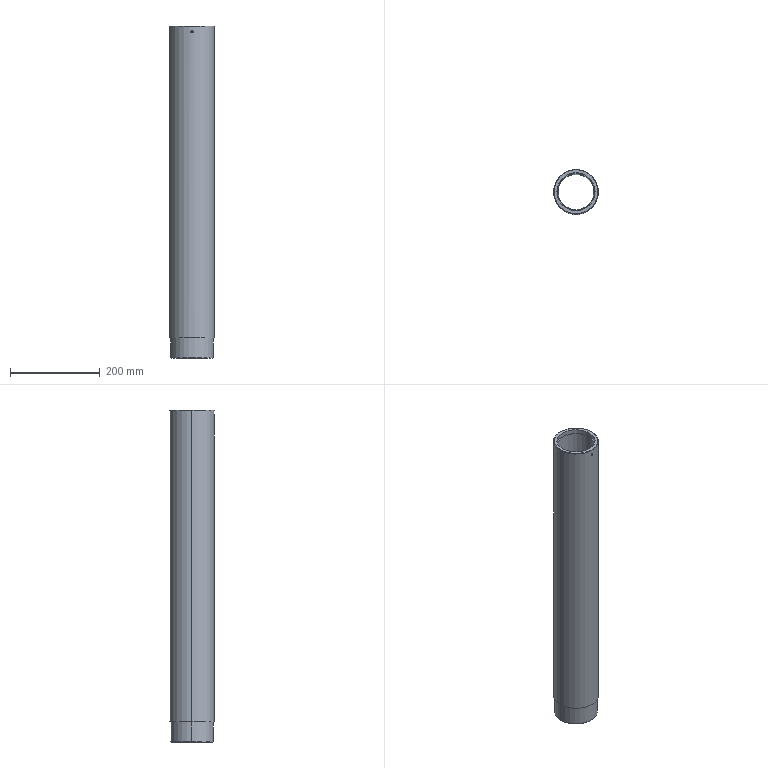Part | SolidWorks | features ICE 6, Chamfer 2, Extrusion 1, HoleWzd 1 | 1 solid | 21 faces | box 100 x 100 x 741 mm | volume 2034515 mm3 | cylinder 12 | plane 5 | cone 4 | commonest cylinder face diameters 5 x2 80 x2 83 x2 85 x2 95 x2 100 x2
STEP:
#1=CARTESIAN_POINT('',(0.,-41.5,730.5));
#2=VERTEX_POINT('',#1);
#3=CARTESIAN_POINT('',(0.,-41.5,725.5));
#4=VERTEX_POINT('',#3);
#5=CARTESIAN_POINT('',(0.,-41.5,730.5));
#6=CARTESIAN_POINT('',(-0.1631,-41.5,730.5));
#7=CARTESIAN_POINT('',(-0.3253,-41.499,730.484));
#8=CARTESIAN_POINT('',(-0.6476,-41.495,730.42));
#9=CARTESIAN_POINT('',(-0.8056,-41.492,730.372));
#10=CARTESIAN_POINT('',(-1.257,-41.482,730.185));
#11=CARTESIAN_POINT('',(-1.536,-41.472,729.999));
#12=CARTESIAN_POINT('',(-1.882,-41.457,729.654));
#13=CARTESIAN_POINT('',(-1.987,-41.452,729.525));
#14=CARTESIAN_POINT('',(-2.169,-41.443,729.254));
#15=CARTESIAN_POINT('',(-2.246,-41.439,729.11));
#16=CARTESIAN_POINT('',(-2.372,-41.432,728.808));
#17=CARTESIAN_POINT('',(-2.42,-41.429,728.649));
#18=CARTESIAN_POINT('',(-2.484,-41.426,728.329));
#19=CARTESIAN_POINT('',(-2.5,-41.425,728.167));
#20=CARTESIAN_POINT('',(-2.5,-41.425,727.837));
#21=CARTESIAN_POINT('',(-2.484,-41.426,727.674));
#22=CARTESIAN_POINT('',(-2.421,-41.429,727.355));
#23=CARTESIAN_POINT('',(-2.373,-41.432,727.196));
#24=CARTESIAN_POINT('',(-2.248,-41.439,726.893));
#25=CARTESIAN_POINT('',(-2.171,-41.443,726.749));
#26=CARTESIAN_POINT('',(-1.99,-41.452,726.478));
#27=CARTESIAN_POINT('',(-1.884,-41.457,726.349));
#28=CARTESIAN_POINT('',(-1.654,-41.467,726.118));
#29=CARTESIAN_POINT('',(-1.528,-41.472,726.015));
#30=CARTESIAN_POINT('',(-1.255,-41.481,725.832));
#31=CARTESIAN_POINT('',(-1.11,-41.485,725.754));
#32=CARTESIAN_POINT('',(-0.6586,-41.496,725.566));
#33=CARTESIAN_POINT('',(-0.3304,-41.5,725.5));
#34=CARTESIAN_POINT('',(0.,-41.5,725.5));
#35=B_SPLINE_CURVE_WITH_KNOTS('',3,(#5,#6,#7,#8,#9,#10,#11,#12,#13,#14,#15,#16,#17,#18,#19,#20,#21,#22,#23,#24,#25,#26,#27,#28,#29,#30,#31,#32,#33,#34),.UNSPECIFIED.,.F.,.F.,(4,2,2,2,2,2,2,2,2,2,2,2,2,2,4),(0.007818,0.008306,0.008795,0.009772,0.01026,0.01075,0.01124,0.01173,0.01221,0.0127,0.01319,0.01368,0.01417,0.01466,0.01563),.UNSPECIFIED.);
#36=EDGE_CURVE('',#2,#4,#35,.T.);
#37=ORIENTED_EDGE('',*,*,#36,.F.);
#38=CARTESIAN_POINT('',(0.,-50.,730.5));
#39=VERTEX_POINT('',#38);
#40=CARTESIAN_POINT('',(0.,-50.,730.5));
#41=DIRECTION('',(0.,-1.,0.));
#42=VECTOR('',#41,1000.);
#43=LINE('',#40,#42);
#44=EDGE_CURVE('',#2,#39,#43,.T.);
#45=ORIENTED_EDGE('',*,*,#44,.T.);
#46=CARTESIAN_POINT('',(0.,-50.,725.5));
#47=VERTEX_POINT('',#46);
#48=CARTESIAN_POINT('',(0.,-50.,725.5));
#49=CARTESIAN_POINT('',(-0.1652,-50.,725.5));
#50=CARTESIAN_POINT('',(-0.3277,-49.999,725.516));
#51=CARTESIAN_POINT('',(-0.6472,-49.996,725.58));
#52=CARTESIAN_POINT('',(-0.806,-49.994,725.628));
#53=CARTESIAN_POINT('',(-1.109,-49.988,725.753));
#54=CARTESIAN_POINT('',(-1.252,-49.984,725.83));
#55=CARTESIAN_POINT('',(-1.524,-49.977,726.012));
#56=CARTESIAN_POINT('',(-1.653,-49.973,726.117));
#57=CARTESIAN_POINT('',(-1.883,-49.965,726.348));
#58=CARTESIAN_POINT('',(-1.987,-49.961,726.474));
#59=CARTESIAN_POINT('',(-2.17,-49.953,726.747));
#60=CARTESIAN_POINT('',(-2.247,-49.95,726.893));
#61=CARTESIAN_POINT('',(-2.372,-49.944,727.193));
#62=CARTESIAN_POINT('',(-2.42,-49.941,727.351));
#63=CARTESIAN_POINT('',(-2.484,-49.938,727.674));
#64=CARTESIAN_POINT('',(-2.5,-49.937,727.836));
#65=CARTESIAN_POINT('',(-2.5,-49.937,728.162));
#66=CARTESIAN_POINT('',(-2.484,-49.938,728.328));
#67=CARTESIAN_POINT('',(-2.42,-49.941,728.649));
#68=CARTESIAN_POINT('',(-2.373,-49.944,728.804));
#69=CARTESIAN_POINT('',(-2.247,-49.95,729.107));
#70=CARTESIAN_POINT('',(-2.169,-49.953,729.253));
#71=CARTESIAN_POINT('',(-1.988,-49.961,729.524));
#72=CARTESIAN_POINT('',(-1.885,-49.965,729.651));
#73=CARTESIAN_POINT('',(-1.651,-49.973,729.884));
#74=CARTESIAN_POINT('',(-1.525,-49.977,729.988));
#75=CARTESIAN_POINT('',(-1.254,-49.984,730.169));
#76=CARTESIAN_POINT('',(-1.108,-49.988,730.247));
#77=CARTESIAN_POINT('',(-0.8052,-49.994,730.372));
#78=CARTESIAN_POINT('',(-0.6493,-49.996,730.42));
#79=CARTESIAN_POINT('',(-0.3289,-49.999,730.484));
#80=CARTESIAN_POINT('',(-0.1632,-50.,730.5));
#81=CARTESIAN_POINT('',(0.,-50.,730.5));
#82=B_SPLINE_CURVE_WITH_KNOTS('',3,(#48,#49,#50,#51,#52,#53,#54,#55,#56,#57,#58,#59,#60,#61,#62,#63,#64,#65,#66,#67,#68,#69,#70,#71,#72,#73,#74,#75,#76,#77,#78,#79,#80,#81),.UNSPECIFIED.,.F.,.F.,(4,2,2,2,2,2,2,2,2,2,2,2,2,2,2,2,4),(0.,0.0004886,0.0009772,0.001466,0.001954,0.002443,0.002932,0.00342,0.003909,0.004397,0.004886,0.005374,0.005863,0.006352,0.00684,0.007329,0.007817),.UNSPECIFIED.);
#83=EDGE_CURVE('',#47,#39,#82,.T.);
#84=ORIENTED_EDGE('',*,*,#83,.F.);
#85=CARTESIAN_POINT('',(0.,-50.,725.5));
#86=DIRECTION('',(0.,-1.,0.));
#87=VECTOR('',#86,1000.);
#88=LINE('',#85,#87);
#89=EDGE_CURVE('',#4,#47,#88,.T.);
#90=ORIENTED_EDGE('',*,*,#89,.F.);
#91=EDGE_LOOP('',(#37,#45,#84,#90));
#92=FACE_OUTER_BOUND('',#91,.T.);
#93=CARTESIAN_POINT('',(0.,-50.,728.));
#94=DIRECTION('',(0.,-1.,0.));
#95=DIRECTION('',(0.,0.,-1.));
#96=AXIS2_PLACEMENT_3D('',#93,#94,#95);
#97=CYLINDRICAL_SURFACE('',#96,2.5);
#98=ADVANCED_FACE('',(#92),#97,.F.);
#99=CARTESIAN_POINT('',(0.,-41.5,725.5));
#100=CARTESIAN_POINT('',(0.1652,-41.5,725.5));
#101=CARTESIAN_POINT('',(0.3277,-41.499,725.516));
#102=CARTESIAN_POINT('',(0.6473,-41.495,725.58));
#103=CARTESIAN_POINT('',(0.8061,-41.492,725.628));
#104=CARTESIAN_POINT('',(1.109,-41.485,725.753));
#105=CARTESIAN_POINT('',(1.252,-41.481,725.83));
#106=CARTESIAN_POINT('',(1.524,-41.472,726.012));
#107=CARTESIAN_POINT('',(1.653,-41.467,726.117));
#108=CARTESIAN_POINT('',(1.883,-41.457,726.348));
#109=CARTESIAN_POINT('',(1.987,-41.453,726.474));
#110=CARTESIAN_POINT('',(2.17,-41.443,726.747));
#111=CARTESIAN_POINT('',(2.247,-41.439,726.893));
#112=CARTESIAN_POINT('',(2.372,-41.432,727.193));
#113=CARTESIAN_POINT('',(2.42,-41.429,727.351));
#114=CARTESIAN_POINT('',(2.484,-41.426,727.674));
#115=CARTESIAN_POINT('',(2.5,-41.425,727.836));
#116=CARTESIAN_POINT('',(2.5,-41.425,728.162));
#117=CARTESIAN_POINT('',(2.484,-41.426,728.328));
#118=CARTESIAN_POINT('',(2.42,-41.429,728.649));
#119=CARTESIAN_POINT('',(2.373,-41.432,728.804));
#120=CARTESIAN_POINT('',(2.247,-41.439,729.107));
#121=CARTESIAN_POINT('',(2.169,-41.443,729.254));
#122=CARTESIAN_POINT('',(1.988,-41.452,729.524));
#123=CARTESIAN_POINT('',(1.885,-41.457,729.651));
#124=CARTESIAN_POINT('',(1.651,-41.467,729.884));
#125=CARTESIAN_POINT('',(1.525,-41.472,729.988));
#126=CARTESIAN_POINT('',(1.254,-41.481,730.169));
#127=CARTESIAN_POINT('',(1.108,-41.485,730.247));
#128=CARTESIAN_POINT('',(0.8052,-41.492,730.372));
#129=CARTESIAN_POINT('',(0.6493,-41.495,730.42));
#130=CARTESIAN_POINT('',(0.3289,-41.499,730.484));
#131=CARTESIAN_POINT('',(0.1632,-41.5,730.5));
#132=CARTESIAN_POINT('',(0.,-41.5,730.5));
#133=B_SPLINE_CURVE_WITH_KNOTS('',3,(#99,#100,#101,#102,#103,#104,#105,#106,#107,#108,#109,#110,#111,#112,#113,#114,#115,#116,#117,#118,#119,#120,#121,#122,#123,#124,#125,#126,#127,#128,#129,#130,#131,#132),.UNSPECIFIED.,.F.,.F.,(4,2,2,2,2,2,2,2,2,2,2,2,2,2,2,2,4),(0.,0.0004886,0.0009772,0.001466,0.001954,0.002443,0.002932,0.00342,0.003909,0.004398,0.004886,0.005375,0.005863,0.006352,0.006841,0.007329,0.007818),.UNSPECIFIED.);
#134=EDGE_CURVE('',#4,#2,#133,.T.);
#135=ORIENTED_EDGE('',*,*,#134,.T.);
#136=ORIENTED_EDGE('',*,*,#36,.T.);
#137=EDGE_LOOP('',(#135,#136));
#138=FACE_BOUND('',#137,.T.);
#139=CARTESIAN_POINT('',(-41.5,0.,681.));
#140=VERTEX_POINT('',#139);
#141=CARTESIAN_POINT('',(41.5,0.,681.));
#142=VERTEX_POINT('',#141);
#143=CARTESIAN_POINT('',(0.,0.,681.));
#144=DIRECTION('',(0.,0.,1.));
#145=DIRECTION('',(1.,0.,0.));
#146=AXIS2_PLACEMENT_3D('',#143,#144,#145);
#147=CIRCLE('',#146,41.5);
#148=EDGE_CURVE('',#140,#142,#147,.T.);
#149=ORIENTED_EDGE('',*,*,#148,.F.);
#150=CARTESIAN_POINT('',(-41.5,0.,731.));
#151=VERTEX_POINT('',#150);
#152=CARTESIAN_POINT('',(-41.5,0.,681.));
#153=DIRECTION('',(0.,0.,1.));
#154=VECTOR('',#153,1000.);
#155=LINE('',#152,#154);
#156=EDGE_CURVE('',#140,#151,#155,.T.);
#157=ORIENTED_EDGE('',*,*,#156,.T.);
#158=CARTESIAN_POINT('',(41.5,0.,731.));
#159=VERTEX_POINT('',#158);
#160=CARTESIAN_POINT('',(0.,0.,731.));
#161=DIRECTION('',(0.,0.,1.));
#162=DIRECTION('',(1.,0.,0.));
#163=AXIS2_PLACEMENT_3D('',#160,#161,#162);
#164=CIRCLE('',#163,41.5);
#165=EDGE_CURVE('',#151,#159,#164,.T.);
#166=ORIENTED_EDGE('',*,*,#165,.T.);
#167=CARTESIAN_POINT('',(41.5,0.,681.));
#168=DIRECTION('',(0.,0.,1.));
#169=VECTOR('',#168,1000.);
#170=LINE('',#167,#169);
#171=EDGE_CURVE('',#142,#159,#170,.T.);
#172=ORIENTED_EDGE('',*,*,#171,.F.);
#173=EDGE_LOOP('',(#149,#157,#166,#172));
#174=FACE_OUTER_BOUND('',#173,.T.);
#175=CARTESIAN_POINT('',(0.,0.,681.));
#176=DIRECTION('',(0.,0.,1.));
#177=DIRECTION('',(1.,0.,0.));
#178=AXIS2_PLACEMENT_3D('',#175,#176,#177);
#179=CYLINDRICAL_SURFACE('',#178,41.5);
#180=ADVANCED_FACE('',(#138,#174),#179,.F.);
#181=CARTESIAN_POINT('',(-42.5,0.,731.));
#182=VERTEX_POINT('',#181);
#183=CARTESIAN_POINT('',(42.5,0.,731.));
#184=VERTEX_POINT('',#183);
#185=CARTESIAN_POINT('',(0.,0.,731.));
#186=DIRECTION('',(0.,0.,1.));
#187=DIRECTION('',(1.,0.,0.));
#188=AXIS2_PLACEMENT_3D('',#185,#186,#187);
#189=CIRCLE('',#188,42.5);
#190=EDGE_CURVE('',#182,#184,#189,.T.);
#191=ORIENTED_EDGE('',*,*,#190,.F.);
#192=CARTESIAN_POINT('',(-42.5,0.,741.));
#193=VERTEX_POINT('',#192);
#194=CARTESIAN_POINT('',(-42.5,0.,731.));
#195=DIRECTION('',(0.,0.,1.));
#196=VECTOR('',#195,1000.);
#197=LINE('',#194,#196);
#198=EDGE_CURVE('',#182,#193,#197,.T.);
#199=ORIENTED_EDGE('',*,*,#198,.T.);
#200=CARTESIAN_POINT('',(42.5,0.,741.));
#201=VERTEX_POINT('',#200);
#202=CARTESIAN_POINT('',(0.,0.,741.));
#203=DIRECTION('',(0.,0.,1.));
#204=DIRECTION('',(1.,0.,0.));
#205=AXIS2_PLACEMENT_3D('',#202,#203,#204);
#206=CIRCLE('',#205,42.5);
#207=EDGE_CURVE('',#193,#201,#206,.T.);
#208=ORIENTED_EDGE('',*,*,#207,.T.);
#209=CARTESIAN_POINT('',(42.5,0.,731.));
#210=DIRECTION('',(0.,0.,1.));
#211=VECTOR('',#210,1000.);
#212=LINE('',#209,#211);
#213=EDGE_CURVE('',#184,#201,#212,.T.);
#214=ORIENTED_EDGE('',*,*,#213,.F.);
#215=EDGE_LOOP('',(#191,#199,#208,#214));
#216=FACE_OUTER_BOUND('',#215,.T.);
#217=CARTESIAN_POINT('',(0.,0.,731.));
#218=DIRECTION('',(0.,0.,1.));
#219=DIRECTION('',(1.,0.,0.));
#220=AXIS2_PLACEMENT_3D('',#217,#218,#219);
#221=CYLINDRICAL_SURFACE('',#220,42.5);
#222=ADVANCED_FACE('',(#216),#221,.F.);
#223=CARTESIAN_POINT('',(49.,0.,741.));
#224=VERTEX_POINT('',#223);
#225=CARTESIAN_POINT('',(-49.,0.,741.));
#226=VERTEX_POINT('',#225);
#227=CARTESIAN_POINT('',(0.,0.,741.));
#228=DIRECTION('',(0.,0.,1.));
#229=DIRECTION('',(1.,0.,0.));
#230=AXIS2_PLACEMENT_3D('',#227,#228,#229);
#231=CIRCLE('',#230,49.);
#232=EDGE_CURVE('',#224,#226,#231,.T.);
#233=ORIENTED_EDGE('',*,*,#232,.F.);
#234=CARTESIAN_POINT('',(50.,0.,740.));
#235=VERTEX_POINT('',#234);
#236=CARTESIAN_POINT('',(49.,0.,741.));
#237=DIRECTION('',(0.7071,0.,-0.7071));
#238=VECTOR('',#237,1000.);
#239=LINE('',#236,#238);
#240=EDGE_CURVE('',#224,#235,#239,.T.);
#241=ORIENTED_EDGE('',*,*,#240,.T.);
#242=CARTESIAN_POINT('',(-50.,0.,740.));
#243=VERTEX_POINT('',#242);
#244=CARTESIAN_POINT('',(0.,0.,740.));
#245=DIRECTION('',(0.,0.,-1.));
#246=DIRECTION('',(1.,0.,0.));
#247=AXIS2_PLACEMENT_3D('',#244,#245,#246);
#248=CIRCLE('',#247,50.);
#249=EDGE_CURVE('',#243,#235,#248,.T.);
#250=ORIENTED_EDGE('',*,*,#249,.F.);
#251=CARTESIAN_POINT('',(-49.,0.,741.));
#252=DIRECTION('',(-0.7071,0.,-0.7071));
#253=VECTOR('',#252,1000.);
#254=LINE('',#251,#253);
#255=EDGE_CURVE('',#226,#243,#254,.T.);
#256=ORIENTED_EDGE('',*,*,#255,.F.);
#257=EDGE_LOOP('',(#233,#241,#250,#256));
#258=FACE_OUTER_BOUND('',#257,.T.);
#259=CARTESIAN_POINT('',(0.,0.,741.));
#260=DIRECTION('',(0.,0.,-1.));
#261=DIRECTION('',(-1.,0.,0.));
#262=AXIS2_PLACEMENT_3D('',#259,#260,#261);
#263=CONICAL_SURFACE('',#262,49.,0.7854);
#264=ADVANCED_FACE('',(#258),#263,.T.);
#265=CARTESIAN_POINT('',(-46.5,0.,0.));
#266=VERTEX_POINT('',#265);
#267=CARTESIAN_POINT('',(46.5,0.,0.));
#268=VERTEX_POINT('',#267);
#269=CARTESIAN_POINT('',(0.,0.,0.));
#270=DIRECTION('',(0.,0.,-1.));
#271=DIRECTION('',(1.,0.,0.));
#272=AXIS2_PLACEMENT_3D('',#269,#270,#271);
#273=CIRCLE('',#272,46.5);
#274=EDGE_CURVE('',#266,#268,#273,.T.);
#275=ORIENTED_EDGE('',*,*,#274,.F.);
#276=CARTESIAN_POINT('',(-47.5,0.,1.));
#277=VERTEX_POINT('',#276);
#278=CARTESIAN_POINT('',(-46.5,0.,0.));
#279=DIRECTION('',(-0.7071,0.,0.7071));
#280=VECTOR('',#279,1000.);
#281=LINE('',#278,#280);
#282=EDGE_CURVE('',#266,#277,#281,.T.);
#283=ORIENTED_EDGE('',*,*,#282,.T.);
#284=CARTESIAN_POINT('',(47.5,0.,1.));
#285=VERTEX_POINT('',#284);
#286=CARTESIAN_POINT('',(0.,0.,1.));
#287=DIRECTION('',(0.,0.,1.));
#288=DIRECTION('',(1.,0.,0.));
#289=AXIS2_PLACEMENT_3D('',#286,#287,#288);
#290=CIRCLE('',#289,47.5);
#291=EDGE_CURVE('',#285,#277,#290,.T.);
#292=ORIENTED_EDGE('',*,*,#291,.F.);
#293=CARTESIAN_POINT('',(46.5,0.,0.));
#294=DIRECTION('',(0.7071,0.,0.7071));
#295=VECTOR('',#294,1000.);
#296=LINE('',#293,#295);
#297=EDGE_CURVE('',#268,#285,#296,.T.);
#298=ORIENTED_EDGE('',*,*,#297,.F.);
#299=EDGE_LOOP('',(#275,#283,#292,#298));
#300=FACE_OUTER_BOUND('',#299,.T.);
#301=CARTESIAN_POINT('',(0.,0.,0.));
#302=DIRECTION('',(0.,0.,1.));
#303=DIRECTION('',(1.,0.,0.));
#304=AXIS2_PLACEMENT_3D('',#301,#302,#303);
#305=CONICAL_SURFACE('',#304,46.5,0.7854);
#306=ADVANCED_FACE('',(#300),#305,.T.);
#307=CARTESIAN_POINT('',(-47.5,0.,45.));
#308=VERTEX_POINT('',#307);
#309=CARTESIAN_POINT('',(47.5,0.,45.));
#310=VERTEX_POINT('',#309);
#311=CARTESIAN_POINT('',(0.,0.,45.));
#312=DIRECTION('',(0.,0.,-1.));
#313=DIRECTION('',(-1.,0.,0.));
#314=AXIS2_PLACEMENT_3D('',#311,#312,#313);
#315=CIRCLE('',#314,47.5);
#316=EDGE_CURVE('',#308,#310,#315,.T.);
#317=ORIENTED_EDGE('',*,*,#316,.T.);
#318=CARTESIAN_POINT('',(47.5,0.,45.));
#319=DIRECTION('',(0.,0.,-1.));
#320=VECTOR('',#319,1000.);
#321=LINE('',#318,#320);
#322=EDGE_CURVE('',#310,#285,#321,.T.);
#323=ORIENTED_EDGE('',*,*,#322,.T.);
#324=ORIENTED_EDGE('',*,*,#291,.T.);
#325=CARTESIAN_POINT('',(-47.5,0.,45.));
#326=DIRECTION('',(0.,0.,-1.));
#327=VECTOR('',#326,1000.);
#328=LINE('',#325,#327);
#329=EDGE_CURVE('',#308,#277,#328,.T.);
#330=ORIENTED_EDGE('',*,*,#329,.F.);
#331=EDGE_LOOP('',(#317,#323,#324,#330));
#332=FACE_OUTER_BOUND('',#331,.T.);
#333=CARTESIAN_POINT('',(0.,0.,45.));
#334=DIRECTION('',(0.,0.,-1.));
#335=DIRECTION('',(-1.,0.,0.));
#336=AXIS2_PLACEMENT_3D('',#333,#334,#335);
#337=CYLINDRICAL_SURFACE('',#336,47.5);
#338=ADVANCED_FACE('',(#332),#337,.T.);
#339=ORIENTED_EDGE('',*,*,#249,.T.);
#340=CARTESIAN_POINT('',(50.,0.,45.));
#341=VERTEX_POINT('',#340);
#342=CARTESIAN_POINT('',(50.,0.,741.));
#343=DIRECTION('',(0.,0.,-1.));
#344=VECTOR('',#343,1000.);
#345=LINE('',#342,#344);
#346=EDGE_CURVE('',#235,#341,#345,.T.);
#347=ORIENTED_EDGE('',*,*,#346,.T.);
#348=CARTESIAN_POINT('',(-50.,0.,45.));
#349=VERTEX_POINT('',#348);
#350=CARTESIAN_POINT('',(0.,0.,45.));
#351=DIRECTION('',(0.,0.,-1.));
#352=DIRECTION('',(-1.,0.,0.));
#353=AXIS2_PLACEMENT_3D('',#350,#351,#352);
#354=CIRCLE('',#353,50.);
#355=EDGE_CURVE('',#349,#341,#354,.T.);
#356=ORIENTED_EDGE('',*,*,#355,.F.);
#357=CARTESIAN_POINT('',(-50.,0.,741.));
#358=DIRECTION('',(0.,0.,-1.));
#359=VECTOR('',#358,1000.);
#360=LINE('',#357,#359);
#361=EDGE_CURVE('',#243,#349,#360,.T.);
#362=ORIENTED_EDGE('',*,*,#361,.F.);
#363=EDGE_LOOP('',(#339,#347,#356,#362));
#364=FACE_OUTER_BOUND('',#363,.T.);
#365=CARTESIAN_POINT('',(0.,0.,741.));
#366=DIRECTION('',(0.,0.,-1.));
#367=DIRECTION('',(-1.,0.,0.));
#368=AXIS2_PLACEMENT_3D('',#365,#366,#367);
#369=CYLINDRICAL_SURFACE('',#368,50.);
#370=ADVANCED_FACE('',(#364),#369,.T.);
#371=CARTESIAN_POINT('',(-40.,0.,681.));
#372=VERTEX_POINT('',#371);
#373=CARTESIAN_POINT('',(40.,0.,681.));
#374=VERTEX_POINT('',#373);
#375=CARTESIAN_POINT('',(0.,0.,681.));
#376=DIRECTION('',(0.,0.,1.));
#377=DIRECTION('',(1.,0.,0.));
#378=AXIS2_PLACEMENT_3D('',#375,#376,#377);
#379=CIRCLE('',#378,40.);
#380=EDGE_CURVE('',#372,#374,#379,.T.);
#381=ORIENTED_EDGE('',*,*,#380,.T.);
#382=CARTESIAN_POINT('',(40.,0.,0.));
#383=VERTEX_POINT('',#382);
#384=CARTESIAN_POINT('',(40.,0.,741.));
#385=DIRECTION('',(0.,0.,-1.));
#386=VECTOR('',#385,1000.);
#387=LINE('',#384,#386);
#388=EDGE_CURVE('',#374,#383,#387,.T.);
#389=ORIENTED_EDGE('',*,*,#388,.T.);
#390=CARTESIAN_POINT('',(-40.,0.,0.));
#391=VERTEX_POINT('',#390);
#392=CARTESIAN_POINT('',(0.,0.,0.));
#393=DIRECTION('',(0.,0.,1.));
#394=DIRECTION('',(1.,0.,0.));
#395=AXIS2_PLACEMENT_3D('',#392,#393,#394);
#396=CIRCLE('',#395,40.);
#397=EDGE_CURVE('',#391,#383,#396,.T.);
#398=ORIENTED_EDGE('',*,*,#397,.F.);
#399=CARTESIAN_POINT('',(-40.,0.,741.));
#400=DIRECTION('',(0.,0.,-1.));
#401=VECTOR('',#400,1000.);
#402=LINE('',#399,#401);
#403=EDGE_CURVE('',#372,#391,#402,.T.);
#404=ORIENTED_EDGE('',*,*,#403,.F.);
#405=EDGE_LOOP('',(#381,#389,#398,#404));
#406=FACE_OUTER_BOUND('',#405,.T.);
#407=CARTESIAN_POINT('',(0.,0.,741.));
#408=DIRECTION('',(0.,0.,-1.));
#409=DIRECTION('',(-1.,0.,0.));
#410=AXIS2_PLACEMENT_3D('',#407,#408,#409);
#411=CYLINDRICAL_SURFACE('',#410,40.);
#412=ADVANCED_FACE('',(#406),#411,.F.);
#413=ORIENTED_EDGE('',*,*,#388,.F.);
#414=CARTESIAN_POINT('',(0.,0.,681.));
#415=DIRECTION('',(0.,0.,1.));
#416=DIRECTION('',(1.,0.,0.));
#417=AXIS2_PLACEMENT_3D('',#414,#415,#416);
#418=CIRCLE('',#417,40.);
#419=EDGE_CURVE('',#374,#372,#418,.T.);
#420=ORIENTED_EDGE('',*,*,#419,.T.);
#421=ORIENTED_EDGE('',*,*,#403,.T.);
#422=CARTESIAN_POINT('',(0.,0.,0.));
#423=DIRECTION('',(0.,0.,1.));
#424=DIRECTION('',(1.,0.,0.));
#425=AXIS2_PLACEMENT_3D('',#422,#423,#424);
#426=CIRCLE('',#425,40.);
#427=EDGE_CURVE('',#383,#391,#426,.T.);
#428=ORIENTED_EDGE('',*,*,#427,.F.);
#429=EDGE_LOOP('',(#413,#420,#421,#428));
#430=FACE_OUTER_BOUND('',#429,.T.);
#431=CARTESIAN_POINT('',(0.,0.,741.));
#432=DIRECTION('',(0.,0.,-1.));
#433=DIRECTION('',(-1.,0.,0.));
#434=AXIS2_PLACEMENT_3D('',#431,#432,#433);
#435=CYLINDRICAL_SURFACE('',#434,40.);
#436=ADVANCED_FACE('',(#430),#435,.F.);
#437=CARTESIAN_POINT('',(0.,0.,0.));
#438=DIRECTION('',(0.,0.,-1.));
#439=DIRECTION('',(1.,0.,0.));
#440=AXIS2_PLACEMENT_3D('',#437,#438,#439);
#441=CIRCLE('',#440,46.5);
#442=EDGE_CURVE('',#268,#266,#441,.T.);
#443=ORIENTED_EDGE('',*,*,#442,.T.);
#444=ORIENTED_EDGE('',*,*,#274,.T.);
#445=EDGE_LOOP('',(#443,#444));
#446=FACE_OUTER_BOUND('',#445,.T.);
#447=ORIENTED_EDGE('',*,*,#397,.T.);
#448=ORIENTED_EDGE('',*,*,#427,.T.);
#449=EDGE_LOOP('',(#447,#448));
#450=FACE_BOUND('',#449,.T.);
#451=CARTESIAN_POINT('',(0.,0.,0.));
#452=DIRECTION('',(0.,0.,1.));
#453=DIRECTION('',(1.,0.,0.));
#454=AXIS2_PLACEMENT_3D('',#451,#452,#453);
#455=PLANE('',#454);
#456=ADVANCED_FACE('',(#446,#450),#455,.F.);
#457=ORIENTED_EDGE('',*,*,#346,.F.);
#458=CARTESIAN_POINT('',(0.,0.,740.));
#459=DIRECTION('',(0.,0.,-1.));
#460=DIRECTION('',(1.,0.,0.));
#461=AXIS2_PLACEMENT_3D('',#458,#459,#460);
#462=CIRCLE('',#461,50.);
#463=EDGE_CURVE('',#235,#243,#462,.T.);
#464=ORIENTED_EDGE('',*,*,#463,.T.);
#465=ORIENTED_EDGE('',*,*,#361,.T.);
#466=CARTESIAN_POINT('',(0.,0.,45.));
#467=DIRECTION('',(0.,0.,-1.));
#468=DIRECTION('',(-1.,0.,0.));
#469=AXIS2_PLACEMENT_3D('',#466,#467,#468);
#470=CIRCLE('',#469,50.);
#471=EDGE_CURVE('',#341,#349,#470,.T.);
#472=ORIENTED_EDGE('',*,*,#471,.F.);
#473=EDGE_LOOP('',(#457,#464,#465,#472));
#474=FACE_OUTER_BOUND('',#473,.T.);
#475=ORIENTED_EDGE('',*,*,#83,.T.);
#476=CARTESIAN_POINT('',(0.,-50.,730.5));
#477=CARTESIAN_POINT('',(0.1631,-50.,730.5));
#478=CARTESIAN_POINT('',(0.3253,-49.999,730.484));
#479=CARTESIAN_POINT('',(0.6476,-49.996,730.42));
#480=CARTESIAN_POINT('',(0.8056,-49.994,730.372));
#481=CARTESIAN_POINT('',(1.257,-49.985,730.185));
#482=CARTESIAN_POINT('',(1.536,-49.977,729.999));
#483=CARTESIAN_POINT('',(1.882,-49.965,729.654));
#484=CARTESIAN_POINT('',(1.987,-49.961,729.525));
#485=CARTESIAN_POINT('',(2.169,-49.953,729.254));
#486=CARTESIAN_POINT('',(2.246,-49.95,729.11));
#487=CARTESIAN_POINT('',(2.372,-49.944,728.808));
#488=CARTESIAN_POINT('',(2.42,-49.941,728.649));
#489=CARTESIAN_POINT('',(2.484,-49.938,728.329));
#490=CARTESIAN_POINT('',(2.5,-49.937,728.167));
#491=CARTESIAN_POINT('',(2.5,-49.937,727.837));
#492=CARTESIAN_POINT('',(2.484,-49.938,727.674));
#493=CARTESIAN_POINT('',(2.421,-49.941,727.355));
#494=CARTESIAN_POINT('',(2.373,-49.944,727.196));
#495=CARTESIAN_POINT('',(2.248,-49.949,726.893));
#496=CARTESIAN_POINT('',(2.171,-49.953,726.749));
#497=CARTESIAN_POINT('',(1.99,-49.96,726.478));
#498=CARTESIAN_POINT('',(1.884,-49.965,726.349));
#499=CARTESIAN_POINT('',(1.654,-49.973,726.118));
#500=CARTESIAN_POINT('',(1.528,-49.977,726.015));
#501=CARTESIAN_POINT('',(1.255,-49.984,725.832));
#502=CARTESIAN_POINT('',(1.11,-49.988,725.754));
#503=CARTESIAN_POINT('',(0.6585,-49.997,725.566));
#504=CARTESIAN_POINT('',(0.3303,-50.,725.5));
#505=CARTESIAN_POINT('',(0.,-50.,725.5));
#506=B_SPLINE_CURVE_WITH_KNOTS('',3,(#476,#477,#478,#479,#480,#481,#482,#483,#484,#485,#486,#487,#488,#489,#490,#491,#492,#493,#494,#495,#496,#497,#498,#499,#500,#501,#502,#503,#504,#505),.UNSPECIFIED.,.F.,.F.,(4,2,2,2,2,2,2,2,2,2,2,2,2,2,4),(0.007817,0.008306,0.008794,0.009771,0.01026,0.01075,0.01124,0.01173,0.01221,0.0127,0.01319,0.01368,0.01417,0.01466,0.01563),.UNSPECIFIED.);
#507=EDGE_CURVE('',#39,#47,#506,.T.);
#508=ORIENTED_EDGE('',*,*,#507,.T.);
#509=EDGE_LOOP('',(#475,#508));
#510=FACE_BOUND('',#509,.T.);
#511=CARTESIAN_POINT('',(0.,0.,741.));
#512=DIRECTION('',(0.,0.,-1.));
#513=DIRECTION('',(-1.,0.,0.));
#514=AXIS2_PLACEMENT_3D('',#511,#512,#513);
#515=CYLINDRICAL_SURFACE('',#514,50.);
#516=ADVANCED_FACE('',(#474,#510),#515,.T.);
#517=CARTESIAN_POINT('',(0.,0.,741.));
#518=DIRECTION('',(0.,0.,1.));
#519=DIRECTION('',(1.,0.,0.));
#520=AXIS2_PLACEMENT_3D('',#517,#518,#519);
#521=CIRCLE('',#520,42.5);
#522=EDGE_CURVE('',#201,#193,#521,.T.);
#523=ORIENTED_EDGE('',*,*,#522,.F.);
#524=ORIENTED_EDGE('',*,*,#207,.F.);
#525=EDGE_LOOP('',(#523,#524));
#526=FACE_BOUND('',#525,.T.);
#527=CARTESIAN_POINT('',(0.,0.,741.));
#528=DIRECTION('',(0.,0.,1.));
#529=DIRECTION('',(1.,0.,0.));
#530=AXIS2_PLACEMENT_3D('',#527,#528,#529);
#531=CIRCLE('',#530,49.);
#532=EDGE_CURVE('',#226,#224,#531,.T.);
#533=ORIENTED_EDGE('',*,*,#532,.T.);
#534=ORIENTED_EDGE('',*,*,#232,.T.);
#535=EDGE_LOOP('',(#533,#534));
#536=FACE_OUTER_BOUND('',#535,.T.);
#537=CARTESIAN_POINT('',(0.,0.,741.));
#538=DIRECTION('',(0.,0.,1.));
#539=DIRECTION('',(1.,0.,0.));
#540=AXIS2_PLACEMENT_3D('',#537,#538,#539);
#541=PLANE('',#540);
#542=ADVANCED_FACE('',(#526,#536),#541,.T.);
#543=ORIENTED_EDGE('',*,*,#316,.F.);
#544=CARTESIAN_POINT('',(0.,0.,45.));
#545=DIRECTION('',(0.,0.,-1.));
#546=DIRECTION('',(-1.,0.,0.));
#547=AXIS2_PLACEMENT_3D('',#544,#545,#546);
#548=CIRCLE('',#547,47.5);
#549=EDGE_CURVE('',#310,#308,#548,.T.);
#550=ORIENTED_EDGE('',*,*,#549,.F.);
#551=EDGE_LOOP('',(#543,#550));
#552=FACE_BOUND('',#551,.T.);
#553=ORIENTED_EDGE('',*,*,#355,.T.);
#554=ORIENTED_EDGE('',*,*,#471,.T.);
#555=EDGE_LOOP('',(#553,#554));
#556=FACE_OUTER_BOUND('',#555,.T.);
#557=CARTESIAN_POINT('',(0.,0.,45.));
#558=DIRECTION('',(0.,0.,-1.));
#559=DIRECTION('',(-1.,0.,0.));
#560=AXIS2_PLACEMENT_3D('',#557,#558,#559);
#561=PLANE('',#560);
#562=ADVANCED_FACE('',(#552,#556),#561,.T.);
#563=ORIENTED_EDGE('',*,*,#322,.F.);
#564=ORIENTED_EDGE('',*,*,#549,.T.);
#565=ORIENTED_EDGE('',*,*,#329,.T.);
#566=CARTESIAN_POINT('',(0.,0.,1.));
#567=DIRECTION('',(0.,0.,1.));
#568=DIRECTION('',(1.,0.,0.));
#569=AXIS2_PLACEMENT_3D('',#566,#567,#568);
#570=CIRCLE('',#569,47.5);
#571=EDGE_CURVE('',#277,#285,#570,.T.);
#572=ORIENTED_EDGE('',*,*,#571,.T.);
#573=EDGE_LOOP('',(#563,#564,#565,#572));
#574=FACE_OUTER_BOUND('',#573,.T.);
#575=CARTESIAN_POINT('',(0.,0.,45.));
#576=DIRECTION('',(0.,0.,-1.));
#577=DIRECTION('',(-1.,0.,0.));
#578=AXIS2_PLACEMENT_3D('',#575,#576,#577);
#579=CYLINDRICAL_SURFACE('',#578,47.5);
#580=ADVANCED_FACE('',(#574),#579,.T.);
#581=ORIENTED_EDGE('',*,*,#282,.F.);
#582=ORIENTED_EDGE('',*,*,#442,.F.);
#583=ORIENTED_EDGE('',*,*,#297,.T.);
#584=ORIENTED_EDGE('',*,*,#571,.F.);
#585=EDGE_LOOP('',(#581,#582,#583,#584));
#586=FACE_OUTER_BOUND('',#585,.T.);
#587=CARTESIAN_POINT('',(0.,0.,0.));
#588=DIRECTION('',(0.,0.,1.));
#589=DIRECTION('',(1.,0.,0.));
#590=AXIS2_PLACEMENT_3D('',#587,#588,#589);
#591=CONICAL_SURFACE('',#590,46.5,0.7854);
#592=ADVANCED_FACE('',(#586),#591,.T.);
#593=ORIENTED_EDGE('',*,*,#240,.F.);
#594=ORIENTED_EDGE('',*,*,#532,.F.);
#595=ORIENTED_EDGE('',*,*,#255,.T.);
#596=ORIENTED_EDGE('',*,*,#463,.F.);
#597=EDGE_LOOP('',(#593,#594,#595,#596));
#598=FACE_OUTER_BOUND('',#597,.T.);
#599=CARTESIAN_POINT('',(0.,0.,741.));
#600=DIRECTION('',(0.,0.,-1.));
#601=DIRECTION('',(-1.,0.,0.));
#602=AXIS2_PLACEMENT_3D('',#599,#600,#601);
#603=CONICAL_SURFACE('',#602,49.,0.7854);
#604=ADVANCED_FACE('',(#598),#603,.T.);
#605=ORIENTED_EDGE('',*,*,#198,.F.);
#606=CARTESIAN_POINT('',(0.,0.,731.));
#607=DIRECTION('',(0.,0.,1.));
#608=DIRECTION('',(1.,0.,0.));
#609=AXIS2_PLACEMENT_3D('',#606,#607,#608);
#610=CIRCLE('',#609,42.5);
#611=EDGE_CURVE('',#184,#182,#610,.T.);
#612=ORIENTED_EDGE('',*,*,#611,.F.);
#613=ORIENTED_EDGE('',*,*,#213,.T.);
#614=ORIENTED_EDGE('',*,*,#522,.T.);
#615=EDGE_LOOP('',(#605,#612,#613,#614));
#616=FACE_OUTER_BOUND('',#615,.T.);
#617=CARTESIAN_POINT('',(0.,0.,731.));
#618=DIRECTION('',(0.,0.,1.));
#619=DIRECTION('',(1.,0.,0.));
#620=AXIS2_PLACEMENT_3D('',#617,#618,#619);
#621=CYLINDRICAL_SURFACE('',#620,42.5);
#622=ADVANCED_FACE('',(#616),#621,.F.);
#623=CARTESIAN_POINT('',(0.,0.,731.));
#624=DIRECTION('',(0.,0.,1.));
#625=DIRECTION('',(1.,0.,0.));
#626=AXIS2_PLACEMENT_3D('',#623,#624,#625);
#627=CIRCLE('',#626,41.5);
#628=EDGE_CURVE('',#159,#151,#627,.T.);
#629=ORIENTED_EDGE('',*,*,#628,.F.);
#630=ORIENTED_EDGE('',*,*,#165,.F.);
#631=EDGE_LOOP('',(#629,#630));
#632=FACE_BOUND('',#631,.T.);
#633=ORIENTED_EDGE('',*,*,#611,.T.);
#634=ORIENTED_EDGE('',*,*,#190,.T.);
#635=EDGE_LOOP('',(#633,#634));
#636=FACE_OUTER_BOUND('',#635,.T.);
#637=CARTESIAN_POINT('',(0.,0.,731.));
#638=DIRECTION('',(0.,0.,1.));
#639=DIRECTION('',(1.,0.,0.));
#640=AXIS2_PLACEMENT_3D('',#637,#638,#639);
#641=PLANE('',#640);
#642=ADVANCED_FACE('',(#632,#636),#641,.T.);
#643=ORIENTED_EDGE('',*,*,#156,.F.);
#644=CARTESIAN_POINT('',(0.,0.,681.));
#645=DIRECTION('',(0.,0.,1.));
#646=DIRECTION('',(1.,0.,0.));
#647=AXIS2_PLACEMENT_3D('',#644,#645,#646);
#648=CIRCLE('',#647,41.5);
#649=EDGE_CURVE('',#142,#140,#648,.T.);
#650=ORIENTED_EDGE('',*,*,#649,.F.);
#651=ORIENTED_EDGE('',*,*,#171,.T.);
#652=ORIENTED_EDGE('',*,*,#628,.T.);
#653=EDGE_LOOP('',(#643,#650,#651,#652));
#654=FACE_OUTER_BOUND('',#653,.T.);
#655=CARTESIAN_POINT('',(0.,0.,681.));
#656=DIRECTION('',(0.,0.,1.));
#657=DIRECTION('',(1.,0.,0.));
#658=AXIS2_PLACEMENT_3D('',#655,#656,#657);
#659=CYLINDRICAL_SURFACE('',#658,41.5);
#660=ADVANCED_FACE('',(#654),#659,.F.);
#661=ORIENTED_EDGE('',*,*,#380,.F.);
#662=ORIENTED_EDGE('',*,*,#419,.F.);
#663=EDGE_LOOP('',(#661,#662));
#664=FACE_BOUND('',#663,.T.);
#665=ORIENTED_EDGE('',*,*,#649,.T.);
#666=ORIENTED_EDGE('',*,*,#148,.T.);
#667=EDGE_LOOP('',(#665,#666));
#668=FACE_OUTER_BOUND('',#667,.T.);
#669=CARTESIAN_POINT('',(0.,0.,681.));
#670=DIRECTION('',(0.,0.,1.));
#671=DIRECTION('',(1.,0.,0.));
#672=AXIS2_PLACEMENT_3D('',#669,#670,#671);
#673=PLANE('',#672);
#674=ADVANCED_FACE('',(#664,#668),#673,.T.);
#675=ORIENTED_EDGE('',*,*,#44,.F.);
#676=ORIENTED_EDGE('',*,*,#134,.F.);
#677=ORIENTED_EDGE('',*,*,#89,.T.);
#678=ORIENTED_EDGE('',*,*,#507,.F.);
#679=EDGE_LOOP('',(#675,#676,#677,#678));
#680=FACE_OUTER_BOUND('',#679,.T.);
#681=CARTESIAN_POINT('',(0.,-50.,728.));
#682=DIRECTION('',(0.,-1.,0.));
#683=DIRECTION('',(0.,0.,-1.));
#684=AXIS2_PLACEMENT_3D('',#681,#682,#683);
#685=CYLINDRICAL_SURFACE('',#684,2.5);
#686=ADVANCED_FACE('',(#680),#685,.F.);
#687=CLOSED_SHELL('',(#98,#180,#222,#264,#306,#338,#370,#412,#436,#456,#516,#542,#562,#580,#592,#604,#622,#642,#660,#674,#686));
#688=MANIFOLD_SOLID_BREP('',#687);
#689=CARTESIAN_POINT('',(0.,0.,0.));
#690=DIRECTION('',(0.,0.,1.));
#691=DIRECTION('',(1.,0.,0.));
#692=AXIS2_PLACEMENT_3D('',#689,#690,#691);
#693=(LENGTH_UNIT()NAMED_UNIT(*)SI_UNIT(.MILLI.,.METRE.));
#694=UNCERTAINTY_MEASURE_WITH_UNIT(LENGTH_MEASURE(0.00001),#693,'','');
#695=(NAMED_UNIT(*)PLANE_ANGLE_UNIT()SI_UNIT($,.RADIAN.));
#696=(NAMED_UNIT(*)SI_UNIT($,.STERADIAN.)SOLID_ANGLE_UNIT());
#697=(GEOMETRIC_REPRESENTATION_CONTEXT(3)GLOBAL_UNCERTAINTY_ASSIGNED_CONTEXT((#694))GLOBAL_UNIT_ASSIGNED_CONTEXT((#693,#695,#696))REPRESENTATION_CONTEXT('',''));
#698=ADVANCED_BREP_SHAPE_REPRESENTATION('',(#688,#692),#697);